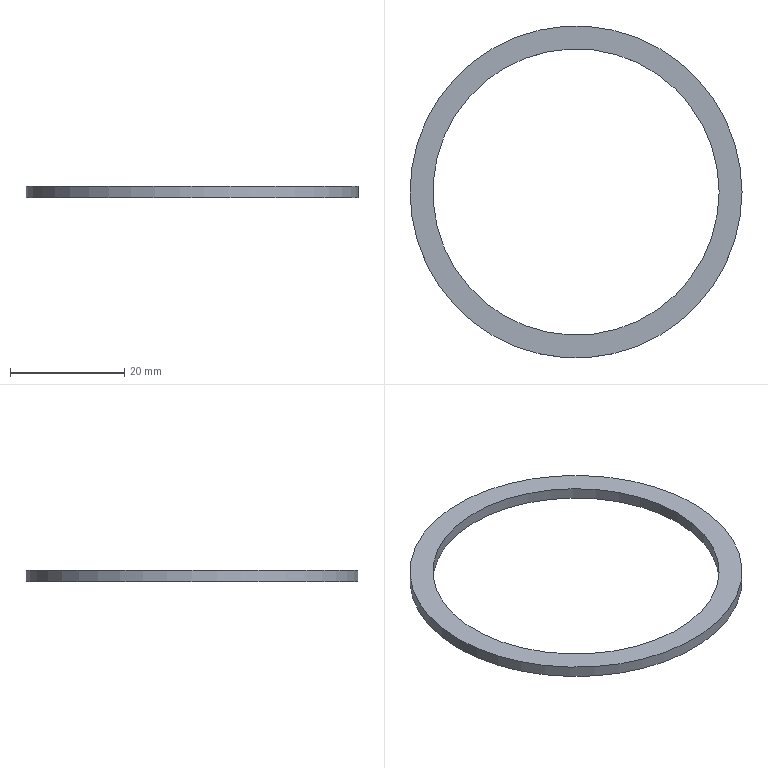Part | NX | features CYLINDER 1, DATUM_CSYS 1, HOLE PACKAGE 1, SIMPLE HOLE 1 | 1 solid | 4 faces | box 58 x 58 x 2 mm | volume 1357 mm3 | plane 2 | cylinder 2 | commonest cylinder face diameters 50 x1 58 x1
STEP:
#1=CARTESIAN_POINT('',(25.,0.,2.));
#2=VERTEX_POINT('',#1);
#3=CARTESIAN_POINT('',(0.,0.,2.));
#4=DIRECTION('',(0.,0.,1.));
#5=DIRECTION('',(1.,0.,0.));
#6=AXIS2_PLACEMENT_3D('',#3,#4,#5);
#7=CIRCLE('',#6,25.);
#8=EDGE_CURVE('',#2,#2,#7,.T.);
#9=ORIENTED_EDGE('',*,*,#8,.F.);
#10=EDGE_LOOP('',(#9));
#11=FACE_BOUND('',#10,.T.);
#12=CARTESIAN_POINT('',(-29.,0.,2.));
#13=VERTEX_POINT('',#12);
#14=CARTESIAN_POINT('',(0.,0.,2.));
#15=DIRECTION('',(0.,0.,-1.));
#16=DIRECTION('',(-1.,0.,0.));
#17=AXIS2_PLACEMENT_3D('',#14,#15,#16);
#18=CIRCLE('',#17,29.);
#19=EDGE_CURVE('',#13,#13,#18,.T.);
#20=ORIENTED_EDGE('',*,*,#19,.F.);
#21=EDGE_LOOP('',(#20));
#22=FACE_BOUND('',#21,.T.);
#23=CARTESIAN_POINT('',(0.,0.,2.));
#24=DIRECTION('',(0.,0.,1.));
#25=DIRECTION('',(1.,0.,0.));
#26=AXIS2_PLACEMENT_3D('',#23,#24,#25);
#27=PLANE('',#26);
#28=ADVANCED_FACE('',(#11,#22),#27,.T.);
#29=CARTESIAN_POINT('',(25.,0.,0.));
#30=VERTEX_POINT('',#29);
#31=CARTESIAN_POINT('',(0.,0.,0.));
#32=DIRECTION('',(0.,0.,1.));
#33=DIRECTION('',(1.,0.,0.));
#34=AXIS2_PLACEMENT_3D('',#31,#32,#33);
#35=CIRCLE('',#34,25.);
#36=EDGE_CURVE('',#30,#30,#35,.T.);
#37=ORIENTED_EDGE('',*,*,#36,.T.);
#38=EDGE_LOOP('',(#37));
#39=FACE_BOUND('',#38,.T.);
#40=CARTESIAN_POINT('',(29.,0.,0.));
#41=VERTEX_POINT('',#40);
#42=CARTESIAN_POINT('',(0.,0.,0.));
#43=DIRECTION('',(0.,0.,1.));
#44=DIRECTION('',(1.,0.,0.));
#45=AXIS2_PLACEMENT_3D('',#42,#43,#44);
#46=CIRCLE('',#45,29.);
#47=EDGE_CURVE('',#41,#41,#46,.T.);
#48=ORIENTED_EDGE('',*,*,#47,.F.);
#49=EDGE_LOOP('',(#48));
#50=FACE_BOUND('',#49,.T.);
#51=CARTESIAN_POINT('',(0.,0.,0.));
#52=DIRECTION('',(0.,0.,-1.));
#53=DIRECTION('',(-1.,0.,0.));
#54=AXIS2_PLACEMENT_3D('',#51,#52,#53);
#55=PLANE('',#54);
#56=ADVANCED_FACE('',(#39,#50),#55,.T.);
#57=ORIENTED_EDGE('',*,*,#19,.T.);
#58=EDGE_LOOP('',(#57));
#59=FACE_BOUND('',#58,.T.);
#60=ORIENTED_EDGE('',*,*,#47,.T.);
#61=EDGE_LOOP('',(#60));
#62=FACE_BOUND('',#61,.T.);
#63=CARTESIAN_POINT('',(0.,0.,0.));
#64=DIRECTION('',(0.,0.,1.));
#65=DIRECTION('',(1.,0.,0.));
#66=AXIS2_PLACEMENT_3D('',#63,#64,#65);
#67=CYLINDRICAL_SURFACE('',#66,29.);
#68=ADVANCED_FACE('',(#59,#62),#67,.T.);
#69=ORIENTED_EDGE('',*,*,#8,.T.);
#70=EDGE_LOOP('',(#69));
#71=FACE_BOUND('',#70,.T.);
#72=ORIENTED_EDGE('',*,*,#36,.F.);
#73=EDGE_LOOP('',(#72));
#74=FACE_BOUND('',#73,.T.);
#75=CARTESIAN_POINT('',(0.,0.,0.));
#76=DIRECTION('',(0.,0.,1.));
#77=DIRECTION('',(1.,0.,0.));
#78=AXIS2_PLACEMENT_3D('',#75,#76,#77);
#79=CYLINDRICAL_SURFACE('',#78,25.);
#80=ADVANCED_FACE('',(#71,#74),#79,.F.);
#81=CLOSED_SHELL('',(#28,#56,#68,#80));
#82=MANIFOLD_SOLID_BREP('',#81);
#83=(LENGTH_UNIT()NAMED_UNIT(*)SI_UNIT(.MILLI.,.METRE.));
#84=UNCERTAINTY_MEASURE_WITH_UNIT(LENGTH_MEASURE(0.00001),#83,'','');
#85=(NAMED_UNIT(*)PLANE_ANGLE_UNIT()SI_UNIT($,.RADIAN.));
#86=(NAMED_UNIT(*)SI_UNIT($,.STERADIAN.)SOLID_ANGLE_UNIT());
#87=(GEOMETRIC_REPRESENTATION_CONTEXT(3)GLOBAL_UNCERTAINTY_ASSIGNED_CONTEXT((#84))GLOBAL_UNIT_ASSIGNED_CONTEXT((#83,#85,#86))REPRESENTATION_CONTEXT('',''));
#88=ADVANCED_BREP_SHAPE_REPRESENTATION('',(#82),#87);